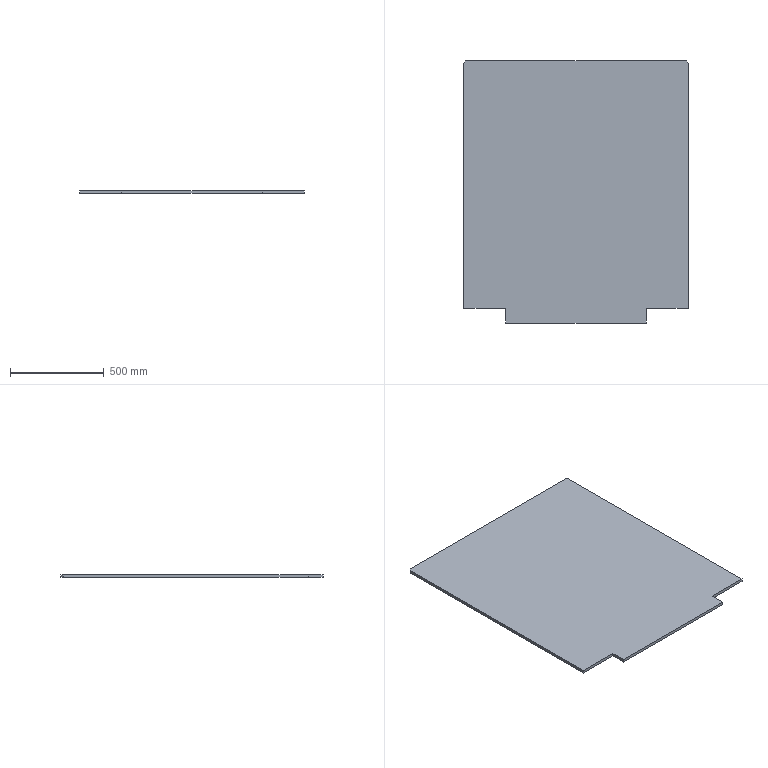Part | SolidWorks | features Chamfer 1, Extrusion 1 | 1 solid | 12 faces | box 1198 x 1399 x 16 mm | volume 26240288 mm3 | plane 12
STEP:
#1=CARTESIAN_POINT('',(-599.,488.,16.));
#2=VERTEX_POINT('',#1);
#3=CARTESIAN_POINT('',(-599.,-819.,16.));
#4=VERTEX_POINT('',#3);
#5=CARTESIAN_POINT('',(-599.,500.,16.));
#6=DIRECTION('',(0.,-1.,0.));
#7=VECTOR('',#6,1000.);
#8=LINE('',#5,#7);
#9=EDGE_CURVE('',#2,#4,#8,.T.);
#10=ORIENTED_EDGE('',*,*,#9,.F.);
#11=CARTESIAN_POINT('',(-599.,488.,0.));
#12=VERTEX_POINT('',#11);
#13=CARTESIAN_POINT('',(-599.,488.,16.));
#14=DIRECTION('',(0.,0.,-1.));
#15=VECTOR('',#14,1000.);
#16=LINE('',#13,#15);
#17=EDGE_CURVE('',#2,#12,#16,.T.);
#18=ORIENTED_EDGE('',*,*,#17,.T.);
#19=CARTESIAN_POINT('',(-599.,-819.,0.));
#20=VERTEX_POINT('',#19);
#21=CARTESIAN_POINT('',(-599.,500.,0.));
#22=DIRECTION('',(0.,-1.,0.));
#23=VECTOR('',#22,1000.);
#24=LINE('',#21,#23);
#25=EDGE_CURVE('',#12,#20,#24,.T.);
#26=ORIENTED_EDGE('',*,*,#25,.T.);
#27=CARTESIAN_POINT('',(-599.,-819.,16.));
#28=DIRECTION('',(0.,0.,-1.));
#29=VECTOR('',#28,1000.);
#30=LINE('',#27,#29);
#31=EDGE_CURVE('',#4,#20,#30,.T.);
#32=ORIENTED_EDGE('',*,*,#31,.F.);
#33=EDGE_LOOP('',(#10,#18,#26,#32));
#34=FACE_OUTER_BOUND('',#33,.T.);
#35=CARTESIAN_POINT('',(-599.,500.,16.));
#36=DIRECTION('',(1.,0.,0.));
#37=DIRECTION('',(0.,1.,0.));
#38=AXIS2_PLACEMENT_3D('',#35,#36,#37);
#39=PLANE('',#38);
#40=ADVANCED_FACE('',(#34),#39,.F.);
#41=CARTESIAN_POINT('',(-375.,-819.,0.));
#42=VERTEX_POINT('',#41);
#43=CARTESIAN_POINT('',(-599.,-819.,0.));
#44=DIRECTION('',(1.,0.,0.));
#45=VECTOR('',#44,1000.);
#46=LINE('',#43,#45);
#47=EDGE_CURVE('',#20,#42,#46,.T.);
#48=ORIENTED_EDGE('',*,*,#47,.T.);
#49=CARTESIAN_POINT('',(-375.,-819.,16.));
#50=VERTEX_POINT('',#49);
#51=CARTESIAN_POINT('',(-375.,-819.,16.));
#52=DIRECTION('',(0.,0.,-1.));
#53=VECTOR('',#52,1000.);
#54=LINE('',#51,#53);
#55=EDGE_CURVE('',#50,#42,#54,.T.);
#56=ORIENTED_EDGE('',*,*,#55,.F.);
#57=CARTESIAN_POINT('',(-599.,-819.,16.));
#58=DIRECTION('',(1.,0.,0.));
#59=VECTOR('',#58,1000.);
#60=LINE('',#57,#59);
#61=EDGE_CURVE('',#4,#50,#60,.T.);
#62=ORIENTED_EDGE('',*,*,#61,.F.);
#63=ORIENTED_EDGE('',*,*,#31,.T.);
#64=EDGE_LOOP('',(#48,#56,#62,#63));
#65=FACE_OUTER_BOUND('',#64,.T.);
#66=CARTESIAN_POINT('',(-599.,-819.,16.));
#67=DIRECTION('',(0.,1.,0.));
#68=DIRECTION('',(0.,0.,1.));
#69=AXIS2_PLACEMENT_3D('',#66,#67,#68);
#70=PLANE('',#69);
#71=ADVANCED_FACE('',(#65),#70,.F.);
#72=CARTESIAN_POINT('',(-375.,-899.,0.));
#73=VERTEX_POINT('',#72);
#74=CARTESIAN_POINT('',(-375.,-819.,0.));
#75=DIRECTION('',(0.,-1.,0.));
#76=VECTOR('',#75,1000.);
#77=LINE('',#74,#76);
#78=EDGE_CURVE('',#42,#73,#77,.T.);
#79=ORIENTED_EDGE('',*,*,#78,.T.);
#80=CARTESIAN_POINT('',(-375.,-899.,16.));
#81=VERTEX_POINT('',#80);
#82=CARTESIAN_POINT('',(-375.,-899.,16.));
#83=DIRECTION('',(0.,0.,-1.));
#84=VECTOR('',#83,1000.);
#85=LINE('',#82,#84);
#86=EDGE_CURVE('',#81,#73,#85,.T.);
#87=ORIENTED_EDGE('',*,*,#86,.F.);
#88=CARTESIAN_POINT('',(-375.,-819.,16.));
#89=DIRECTION('',(0.,-1.,0.));
#90=VECTOR('',#89,1000.);
#91=LINE('',#88,#90);
#92=EDGE_CURVE('',#50,#81,#91,.T.);
#93=ORIENTED_EDGE('',*,*,#92,.F.);
#94=ORIENTED_EDGE('',*,*,#55,.T.);
#95=EDGE_LOOP('',(#79,#87,#93,#94));
#96=FACE_OUTER_BOUND('',#95,.T.);
#97=CARTESIAN_POINT('',(-375.,-819.,16.));
#98=DIRECTION('',(1.,0.,0.));
#99=DIRECTION('',(0.,0.,-1.));
#100=AXIS2_PLACEMENT_3D('',#97,#98,#99);
#101=PLANE('',#100);
#102=ADVANCED_FACE('',(#96),#101,.F.);
#103=CARTESIAN_POINT('',(375.,-899.,0.));
#104=VERTEX_POINT('',#103);
#105=CARTESIAN_POINT('',(-375.,-899.,0.));
#106=DIRECTION('',(1.,0.,0.));
#107=VECTOR('',#106,1000.);
#108=LINE('',#105,#107);
#109=EDGE_CURVE('',#73,#104,#108,.T.);
#110=ORIENTED_EDGE('',*,*,#109,.T.);
#111=CARTESIAN_POINT('',(375.,-899.,16.));
#112=VERTEX_POINT('',#111);
#113=CARTESIAN_POINT('',(375.,-899.,16.));
#114=DIRECTION('',(0.,0.,-1.));
#115=VECTOR('',#114,1000.);
#116=LINE('',#113,#115);
#117=EDGE_CURVE('',#112,#104,#116,.T.);
#118=ORIENTED_EDGE('',*,*,#117,.F.);
#119=CARTESIAN_POINT('',(-375.,-899.,16.));
#120=DIRECTION('',(1.,0.,0.));
#121=VECTOR('',#120,1000.);
#122=LINE('',#119,#121);
#123=EDGE_CURVE('',#81,#112,#122,.T.);
#124=ORIENTED_EDGE('',*,*,#123,.F.);
#125=ORIENTED_EDGE('',*,*,#86,.T.);
#126=EDGE_LOOP('',(#110,#118,#124,#125));
#127=FACE_OUTER_BOUND('',#126,.T.);
#128=CARTESIAN_POINT('',(-375.,-899.,16.));
#129=DIRECTION('',(0.,1.,0.));
#130=DIRECTION('',(0.,0.,1.));
#131=AXIS2_PLACEMENT_3D('',#128,#129,#130);
#132=PLANE('',#131);
#133=ADVANCED_FACE('',(#127),#132,.F.);
#134=CARTESIAN_POINT('',(375.,-819.,0.));
#135=VERTEX_POINT('',#134);
#136=CARTESIAN_POINT('',(375.,-899.,0.));
#137=DIRECTION('',(0.,1.,0.));
#138=VECTOR('',#137,1000.);
#139=LINE('',#136,#138);
#140=EDGE_CURVE('',#104,#135,#139,.T.);
#141=ORIENTED_EDGE('',*,*,#140,.T.);
#142=CARTESIAN_POINT('',(375.,-819.,16.));
#143=VERTEX_POINT('',#142);
#144=CARTESIAN_POINT('',(375.,-819.,16.));
#145=DIRECTION('',(0.,0.,-1.));
#146=VECTOR('',#145,1000.);
#147=LINE('',#144,#146);
#148=EDGE_CURVE('',#143,#135,#147,.T.);
#149=ORIENTED_EDGE('',*,*,#148,.F.);
#150=CARTESIAN_POINT('',(375.,-899.,16.));
#151=DIRECTION('',(0.,1.,0.));
#152=VECTOR('',#151,1000.);
#153=LINE('',#150,#152);
#154=EDGE_CURVE('',#112,#143,#153,.T.);
#155=ORIENTED_EDGE('',*,*,#154,.F.);
#156=ORIENTED_EDGE('',*,*,#117,.T.);
#157=EDGE_LOOP('',(#141,#149,#155,#156));
#158=FACE_OUTER_BOUND('',#157,.T.);
#159=CARTESIAN_POINT('',(375.,-899.,16.));
#160=DIRECTION('',(-1.,0.,0.));
#161=DIRECTION('',(0.,0.,1.));
#162=AXIS2_PLACEMENT_3D('',#159,#160,#161);
#163=PLANE('',#162);
#164=ADVANCED_FACE('',(#158),#163,.F.);
#165=CARTESIAN_POINT('',(599.,-819.,0.));
#166=VERTEX_POINT('',#165);
#167=CARTESIAN_POINT('',(375.,-819.,0.));
#168=DIRECTION('',(1.,0.,0.));
#169=VECTOR('',#168,1000.);
#170=LINE('',#167,#169);
#171=EDGE_CURVE('',#135,#166,#170,.T.);
#172=ORIENTED_EDGE('',*,*,#171,.T.);
#173=CARTESIAN_POINT('',(599.,-819.,16.));
#174=VERTEX_POINT('',#173);
#175=CARTESIAN_POINT('',(599.,-819.,16.));
#176=DIRECTION('',(0.,0.,-1.));
#177=VECTOR('',#176,1000.);
#178=LINE('',#175,#177);
#179=EDGE_CURVE('',#174,#166,#178,.T.);
#180=ORIENTED_EDGE('',*,*,#179,.F.);
#181=CARTESIAN_POINT('',(375.,-819.,16.));
#182=DIRECTION('',(1.,0.,0.));
#183=VECTOR('',#182,1000.);
#184=LINE('',#181,#183);
#185=EDGE_CURVE('',#143,#174,#184,.T.);
#186=ORIENTED_EDGE('',*,*,#185,.F.);
#187=ORIENTED_EDGE('',*,*,#148,.T.);
#188=EDGE_LOOP('',(#172,#180,#186,#187));
#189=FACE_OUTER_BOUND('',#188,.T.);
#190=CARTESIAN_POINT('',(375.,-819.,16.));
#191=DIRECTION('',(0.,1.,0.));
#192=DIRECTION('',(-1.,0.,0.));
#193=AXIS2_PLACEMENT_3D('',#190,#191,#192);
#194=PLANE('',#193);
#195=ADVANCED_FACE('',(#189),#194,.F.);
#196=CARTESIAN_POINT('',(599.,488.,0.));
#197=VERTEX_POINT('',#196);
#198=CARTESIAN_POINT('',(599.,500.,0.));
#199=DIRECTION('',(0.,1.,0.));
#200=VECTOR('',#199,1000.);
#201=LINE('',#198,#200);
#202=EDGE_CURVE('',#166,#197,#201,.T.);
#203=ORIENTED_EDGE('',*,*,#202,.T.);
#204=CARTESIAN_POINT('',(599.,488.,16.));
#205=VERTEX_POINT('',#204);
#206=CARTESIAN_POINT('',(599.,488.,16.));
#207=DIRECTION('',(0.,0.,1.));
#208=VECTOR('',#207,1000.);
#209=LINE('',#206,#208);
#210=EDGE_CURVE('',#197,#205,#209,.T.);
#211=ORIENTED_EDGE('',*,*,#210,.T.);
#212=CARTESIAN_POINT('',(599.,500.,16.));
#213=DIRECTION('',(0.,1.,0.));
#214=VECTOR('',#213,1000.);
#215=LINE('',#212,#214);
#216=EDGE_CURVE('',#174,#205,#215,.T.);
#217=ORIENTED_EDGE('',*,*,#216,.F.);
#218=ORIENTED_EDGE('',*,*,#179,.T.);
#219=EDGE_LOOP('',(#203,#211,#217,#218));
#220=FACE_OUTER_BOUND('',#219,.T.);
#221=CARTESIAN_POINT('',(599.,500.,16.));
#222=DIRECTION('',(-1.,0.,0.));
#223=DIRECTION('',(0.,0.,1.));
#224=AXIS2_PLACEMENT_3D('',#221,#222,#223);
#225=PLANE('',#224);
#226=ADVANCED_FACE('',(#220),#225,.F.);
#227=CARTESIAN_POINT('',(587.,500.,16.));
#228=VERTEX_POINT('',#227);
#229=CARTESIAN_POINT('',(-587.,500.,16.));
#230=VERTEX_POINT('',#229);
#231=CARTESIAN_POINT('',(599.,500.,16.));
#232=DIRECTION('',(-1.,0.,0.));
#233=VECTOR('',#232,1000.);
#234=LINE('',#231,#233);
#235=EDGE_CURVE('',#228,#230,#234,.T.);
#236=ORIENTED_EDGE('',*,*,#235,.F.);
#237=CARTESIAN_POINT('',(587.,500.,0.));
#238=VERTEX_POINT('',#237);
#239=CARTESIAN_POINT('',(587.,500.,16.));
#240=DIRECTION('',(0.,0.,-1.));
#241=VECTOR('',#240,1000.);
#242=LINE('',#239,#241);
#243=EDGE_CURVE('',#228,#238,#242,.T.);
#244=ORIENTED_EDGE('',*,*,#243,.T.);
#245=CARTESIAN_POINT('',(-587.,500.,0.));
#246=VERTEX_POINT('',#245);
#247=CARTESIAN_POINT('',(599.,500.,0.));
#248=DIRECTION('',(-1.,0.,0.));
#249=VECTOR('',#248,1000.);
#250=LINE('',#247,#249);
#251=EDGE_CURVE('',#238,#246,#250,.T.);
#252=ORIENTED_EDGE('',*,*,#251,.T.);
#253=CARTESIAN_POINT('',(-587.,500.,16.));
#254=DIRECTION('',(0.,0.,1.));
#255=VECTOR('',#254,1000.);
#256=LINE('',#253,#255);
#257=EDGE_CURVE('',#246,#230,#256,.T.);
#258=ORIENTED_EDGE('',*,*,#257,.T.);
#259=EDGE_LOOP('',(#236,#244,#252,#258));
#260=FACE_OUTER_BOUND('',#259,.T.);
#261=CARTESIAN_POINT('',(599.,500.,16.));
#262=DIRECTION('',(0.,-1.,0.));
#263=DIRECTION('',(1.,0.,0.));
#264=AXIS2_PLACEMENT_3D('',#261,#262,#263);
#265=PLANE('',#264);
#266=ADVANCED_FACE('',(#260),#265,.F.);
#267=ORIENTED_EDGE('',*,*,#216,.T.);
#268=CARTESIAN_POINT('',(543.5,543.5,16.));
#269=DIRECTION('',(-0.7071,0.7071,0.));
#270=VECTOR('',#269,1000.);
#271=LINE('',#268,#270);
#272=EDGE_CURVE('',#205,#228,#271,.T.);
#273=ORIENTED_EDGE('',*,*,#272,.T.);
#274=ORIENTED_EDGE('',*,*,#235,.T.);
#275=CARTESIAN_POINT('',(-543.5,543.5,16.));
#276=DIRECTION('',(-0.7071,-0.7071,0.));
#277=VECTOR('',#276,1000.);
#278=LINE('',#275,#277);
#279=EDGE_CURVE('',#230,#2,#278,.T.);
#280=ORIENTED_EDGE('',*,*,#279,.T.);
#281=ORIENTED_EDGE('',*,*,#9,.T.);
#282=ORIENTED_EDGE('',*,*,#61,.T.);
#283=ORIENTED_EDGE('',*,*,#92,.T.);
#284=ORIENTED_EDGE('',*,*,#123,.T.);
#285=ORIENTED_EDGE('',*,*,#154,.T.);
#286=ORIENTED_EDGE('',*,*,#185,.T.);
#287=EDGE_LOOP('',(#267,#273,#274,#280,#281,#282,#283,#284,#285,#286));
#288=FACE_OUTER_BOUND('',#287,.T.);
#289=CARTESIAN_POINT('',(0.,0.,16.));
#290=DIRECTION('',(0.,0.,1.));
#291=DIRECTION('',(1.,0.,0.));
#292=AXIS2_PLACEMENT_3D('',#289,#290,#291);
#293=PLANE('',#292);
#294=ADVANCED_FACE('',(#288),#293,.T.);
#295=ORIENTED_EDGE('',*,*,#251,.F.);
#296=CARTESIAN_POINT('',(587.,500.,0.));
#297=DIRECTION('',(0.7071,-0.7071,0.));
#298=VECTOR('',#297,1000.);
#299=LINE('',#296,#298);
#300=EDGE_CURVE('',#238,#197,#299,.T.);
#301=ORIENTED_EDGE('',*,*,#300,.T.);
#302=ORIENTED_EDGE('',*,*,#202,.F.);
#303=ORIENTED_EDGE('',*,*,#171,.F.);
#304=ORIENTED_EDGE('',*,*,#140,.F.);
#305=ORIENTED_EDGE('',*,*,#109,.F.);
#306=ORIENTED_EDGE('',*,*,#78,.F.);
#307=ORIENTED_EDGE('',*,*,#47,.F.);
#308=ORIENTED_EDGE('',*,*,#25,.F.);
#309=CARTESIAN_POINT('',(-599.,488.,0.));
#310=DIRECTION('',(0.7071,0.7071,0.));
#311=VECTOR('',#310,1000.);
#312=LINE('',#309,#311);
#313=EDGE_CURVE('',#12,#246,#312,.T.);
#314=ORIENTED_EDGE('',*,*,#313,.T.);
#315=EDGE_LOOP('',(#295,#301,#302,#303,#304,#305,#306,#307,#308,#314));
#316=FACE_OUTER_BOUND('',#315,.T.);
#317=CARTESIAN_POINT('',(0.,0.,0.));
#318=DIRECTION('',(0.,0.,1.));
#319=DIRECTION('',(1.,0.,0.));
#320=AXIS2_PLACEMENT_3D('',#317,#318,#319);
#321=PLANE('',#320);
#322=ADVANCED_FACE('',(#316),#321,.F.);
#323=ORIENTED_EDGE('',*,*,#272,.F.);
#324=ORIENTED_EDGE('',*,*,#210,.F.);
#325=ORIENTED_EDGE('',*,*,#300,.F.);
#326=ORIENTED_EDGE('',*,*,#243,.F.);
#327=EDGE_LOOP('',(#323,#324,#325,#326));
#328=FACE_OUTER_BOUND('',#327,.T.);
#329=CARTESIAN_POINT('',(587.,500.,16.));
#330=DIRECTION('',(-0.7071,-0.7071,0.));
#331=DIRECTION('',(0.,0.,-1.));
#332=AXIS2_PLACEMENT_3D('',#329,#330,#331);
#333=PLANE('',#332);
#334=ADVANCED_FACE('',(#328),#333,.F.);
#335=ORIENTED_EDGE('',*,*,#279,.F.);
#336=ORIENTED_EDGE('',*,*,#257,.F.);
#337=ORIENTED_EDGE('',*,*,#313,.F.);
#338=ORIENTED_EDGE('',*,*,#17,.F.);
#339=EDGE_LOOP('',(#335,#336,#337,#338));
#340=FACE_OUTER_BOUND('',#339,.T.);
#341=CARTESIAN_POINT('',(-599.,488.,16.));
#342=DIRECTION('',(0.7071,-0.7071,0.));
#343=DIRECTION('',(0.,0.,-1.));
#344=AXIS2_PLACEMENT_3D('',#341,#342,#343);
#345=PLANE('',#344);
#346=ADVANCED_FACE('',(#340),#345,.F.);
#347=CLOSED_SHELL('',(#40,#71,#102,#133,#164,#195,#226,#266,#294,#322,#334,#346));
#348=MANIFOLD_SOLID_BREP('',#347);
#349=CARTESIAN_POINT('',(0.,0.,0.));
#350=DIRECTION('',(0.,0.,1.));
#351=DIRECTION('',(1.,0.,0.));
#352=AXIS2_PLACEMENT_3D('',#349,#350,#351);
#353=(LENGTH_UNIT()NAMED_UNIT(*)SI_UNIT(.MILLI.,.METRE.));
#354=UNCERTAINTY_MEASURE_WITH_UNIT(LENGTH_MEASURE(0.00001),#353,'','');
#355=(NAMED_UNIT(*)PLANE_ANGLE_UNIT()SI_UNIT($,.RADIAN.));
#356=(NAMED_UNIT(*)SI_UNIT($,.STERADIAN.)SOLID_ANGLE_UNIT());
#357=(GEOMETRIC_REPRESENTATION_CONTEXT(3)GLOBAL_UNCERTAINTY_ASSIGNED_CONTEXT((#354))GLOBAL_UNIT_ASSIGNED_CONTEXT((#353,#355,#356))REPRESENTATION_CONTEXT('',''));
#358=ADVANCED_BREP_SHAPE_REPRESENTATION('',(#348,#352),#357);